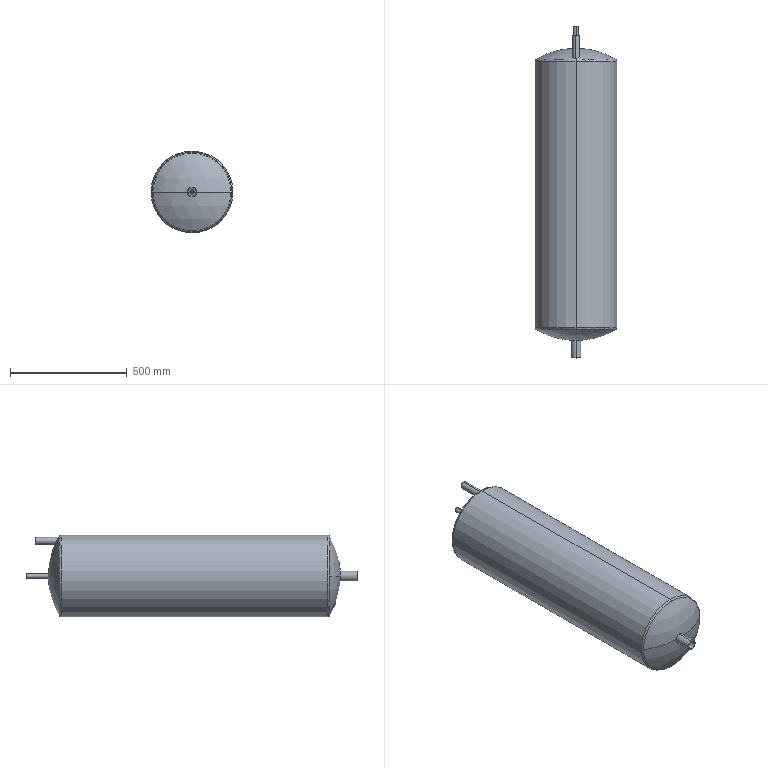Part | SolidWorks | features ICE 8, Revolution 1 | 1 solid | 35 faces | box 350 x 1420 x 350 mm | volume 7280812 mm3 | cylinder 16 | torus 8 | sphere 8 | plane 3 | commonest cylinder face diameters 10 x2 20 x2 26 x2 30 x2 37 x2 42 x2
STEP:
#1=CARTESIAN_POINT('',(0.,576.425,163.));
#2=VERTEX_POINT('',#1);
#3=CARTESIAN_POINT('',(0.,589.882,137.));
#4=VERTEX_POINT('',#3);
#5=CARTESIAN_POINT('',(0.,576.425,163.));
#6=CARTESIAN_POINT('',(-0.4541,576.425,163.));
#7=CARTESIAN_POINT('',(-0.9133,576.438,162.976));
#8=CARTESIAN_POINT('',(-1.814,576.488,162.881));
#9=CARTESIAN_POINT('',(-2.259,576.525,162.81));
#10=CARTESIAN_POINT('',(-3.136,576.624,162.624));
#11=CARTESIAN_POINT('',(-3.569,576.685,162.508));
#12=CARTESIAN_POINT('',(-4.425,576.831,162.232));
#13=CARTESIAN_POINT('',(-4.846,576.917,162.071));
#14=CARTESIAN_POINT('',(-6.062,577.201,161.534));
#15=CARTESIAN_POINT('',(-6.822,577.43,161.101));
#16=CARTESIAN_POINT('',(-7.888,577.829,160.343));
#17=CARTESIAN_POINT('',(-8.229,577.971,160.073));
#18=CARTESIAN_POINT('',(-8.873,578.268,159.51));
#19=CARTESIAN_POINT('',(-9.179,578.423,159.216));
#20=CARTESIAN_POINT('',(-9.757,578.746,158.601));
#21=CARTESIAN_POINT('',(-10.03,578.915,158.281));
#22=CARTESIAN_POINT('',(-10.544,579.264,157.616));
#23=CARTESIAN_POINT('',(-10.784,579.445,157.271));
#24=CARTESIAN_POINT('',(-11.446,579.996,156.219));
#25=CARTESIAN_POINT('',(-11.813,580.378,155.488));
#26=CARTESIAN_POINT('',(-12.258,580.972,154.349));
#27=CARTESIAN_POINT('',(-12.388,581.175,153.961));
#28=CARTESIAN_POINT('',(-12.612,581.582,153.179));
#29=CARTESIAN_POINT('',(-12.704,581.787,152.785));
#30=CARTESIAN_POINT('',(-12.926,582.403,151.6));
#31=CARTESIAN_POINT('',(-13.,582.817,150.802));
#32=CARTESIAN_POINT('',(-13.,583.442,149.594));
#33=CARTESIAN_POINT('',(-12.981,583.651,149.188));
#34=CARTESIAN_POINT('',(-12.905,584.067,148.382));
#35=CARTESIAN_POINT('',(-12.849,584.274,147.982));
#36=CARTESIAN_POINT('',(-12.698,584.684,147.187));
#37=CARTESIAN_POINT('',(-12.605,584.887,146.792));
#38=CARTESIAN_POINT('',(-12.378,585.29,146.007));
#39=CARTESIAN_POINT('',(-12.246,585.49,145.619));
#40=CARTESIAN_POINT('',(-11.799,586.074,144.481));
#41=CARTESIAN_POINT('',(-11.43,586.447,143.751));
#42=CARTESIAN_POINT('',(-10.766,586.984,142.702));
#43=CARTESIAN_POINT('',(-10.527,587.158,142.36));
#44=CARTESIAN_POINT('',(-10.008,587.499,141.692));
#45=CARTESIAN_POINT('',(-9.733,587.662,141.372));
#46=CARTESIAN_POINT('',(-8.863,588.131,140.452));
#47=CARTESIAN_POINT('',(-8.222,588.415,139.893));
#48=CARTESIAN_POINT('',(-7.162,588.797,139.142));
#49=CARTESIAN_POINT('',(-6.79,588.917,138.906));
#50=CARTESIAN_POINT('',(-6.023,589.137,138.471));
#51=CARTESIAN_POINT('',(-5.629,589.237,138.274));
#52=CARTESIAN_POINT('',(-4.42,589.506,137.743));
#53=CARTESIAN_POINT('',(-3.575,589.645,137.469));
#54=CARTESIAN_POINT('',(-2.246,589.787,137.188));
#55=CARTESIAN_POINT('',(-1.796,589.823,137.117));
#56=CARTESIAN_POINT('',(-0.8995,589.87,137.023));
#57=CARTESIAN_POINT('',(-0.4502,589.882,137.));
#58=CARTESIAN_POINT('',(0.,589.882,137.));
#59=B_SPLINE_CURVE_WITH_KNOTS('',3,(#5,#6,#7,#8,#9,#10,#11,#12,#13,#14,#15,#16,#17,#18,#19,#20,#21,#22,#23,#24,#25,#26,#27,#28,#29,#30,#31,#32,#33,#34,#35,#36,#37,#38,#39,#40,#41,#42,#43,#44,#45,#46,#47,#48,#49,#50,#51,#52,#53,#54,#55,#56,#57,#58),.UNSPECIFIED.,.F.,.F.,(4,2,2,2,2,2,2,2,2,2,2,2,2,2,2,2,2,2,2,2,2,2,2,2,2,2,4),(0.06034,0.06169,0.06303,0.06438,0.06573,0.06843,0.06978,0.07112,0.07247,0.07382,0.07652,0.07787,0.07921,0.08191,0.08326,0.08461,0.08596,0.08731,0.09,0.09135,0.0927,0.0954,0.09674,0.09809,0.1008,0.1021,0.1035),.UNSPECIFIED.);
#60=EDGE_CURVE('',#2,#4,#59,.T.);
#61=ORIENTED_EDGE('',*,*,#60,.T.);
#62=CARTESIAN_POINT('',(0.,680.,137.));
#63=VERTEX_POINT('',#62);
#64=CARTESIAN_POINT('',(0.,-700.001,137.));
#65=DIRECTION('',(0.,1.,0.));
#66=VECTOR('',#65,1000.);
#67=LINE('',#64,#66);
#68=EDGE_CURVE('',#4,#63,#67,.T.);
#69=ORIENTED_EDGE('',*,*,#68,.T.);
#70=CARTESIAN_POINT('',(0.,680.,163.));
#71=VERTEX_POINT('',#70);
#72=CARTESIAN_POINT('',(0.,680.,150.));
#73=DIRECTION('',(0.,1.,0.));
#74=DIRECTION('',(0.,0.,1.));
#75=AXIS2_PLACEMENT_3D('',#72,#73,#74);
#76=CIRCLE('',#75,13.);
#77=EDGE_CURVE('',#63,#71,#76,.T.);
#78=ORIENTED_EDGE('',*,*,#77,.T.);
#79=CARTESIAN_POINT('',(0.,-700.001,163.));
#80=DIRECTION('',(0.,1.,0.));
#81=VECTOR('',#80,1000.);
#82=LINE('',#79,#81);
#83=EDGE_CURVE('',#2,#71,#82,.T.);
#84=ORIENTED_EDGE('',*,*,#83,.F.);
#85=EDGE_LOOP('',(#61,#69,#78,#84));
#86=FACE_OUTER_BOUND('',#85,.T.);
#87=CARTESIAN_POINT('',(0.,-700.001,150.));
#88=DIRECTION('',(0.,1.,0.));
#89=DIRECTION('',(0.,0.,1.));
#90=AXIS2_PLACEMENT_3D('',#87,#88,#89);
#91=CYLINDRICAL_SURFACE('',#90,13.);
#92=ADVANCED_FACE('',(#86),#91,.F.);
#93=CARTESIAN_POINT('',(0.,581.042,165.));
#94=VERTEX_POINT('',#93);
#95=CARTESIAN_POINT('',(0.,596.28,135.));
#96=VERTEX_POINT('',#95);
#97=CARTESIAN_POINT('',(0.,581.042,165.));
#98=CARTESIAN_POINT('',(1.049,581.042,165.));
#99=CARTESIAN_POINT('',(2.08,581.099,164.891));
#100=CARTESIAN_POINT('',(3.602,581.266,164.57));
#101=CARTESIAN_POINT('',(4.108,581.336,164.436));
#102=CARTESIAN_POINT('',(5.093,581.502,164.118));
#103=CARTESIAN_POINT('',(5.572,581.597,163.936));
#104=CARTESIAN_POINT('',(6.504,581.81,163.526));
#105=CARTESIAN_POINT('',(6.957,581.928,163.299));
#106=CARTESIAN_POINT('',(7.837,582.187,162.8));
#107=CARTESIAN_POINT('',(8.267,582.329,162.526));
#108=CARTESIAN_POINT('',(9.493,582.78,161.657));
#109=CARTESIAN_POINT('',(10.235,583.116,161.009));
#110=CARTESIAN_POINT('',(11.242,583.667,159.943));
#111=CARTESIAN_POINT('',(11.561,583.86,159.57));
#112=CARTESIAN_POINT('',(12.154,584.255,158.804));
#113=CARTESIAN_POINT('',(12.429,584.458,158.41));
#114=CARTESIAN_POINT('',(13.193,585.08,157.201));
#115=CARTESIAN_POINT('',(13.62,585.515,156.356));
#116=CARTESIAN_POINT('',(14.312,586.42,154.59));
#117=CARTESIAN_POINT('',(14.568,586.879,153.692));
#118=CARTESIAN_POINT('',(14.826,587.577,152.324));
#119=CARTESIAN_POINT('',(14.891,587.811,151.864));
#120=CARTESIAN_POINT('',(14.978,588.283,150.938));
#121=CARTESIAN_POINT('',(15.,588.521,150.47));
#122=CARTESIAN_POINT('',(15.,589.232,149.069));
#123=CARTESIAN_POINT('',(14.914,589.7,148.146));
#124=CARTESIAN_POINT('',(14.657,590.391,146.778));
#125=CARTESIAN_POINT('',(14.55,590.62,146.325));
#126=CARTESIAN_POINT('',(14.292,591.074,145.423));
#127=CARTESIAN_POINT('',(14.141,591.301,144.974));
#128=CARTESIAN_POINT('',(13.622,591.968,143.648));
#129=CARTESIAN_POINT('',(13.195,592.392,142.804));
#130=CARTESIAN_POINT('',(12.433,592.997,141.595));
#131=CARTESIAN_POINT('',(12.159,593.194,141.202));
#132=CARTESIAN_POINT('',(11.566,593.576,140.437));
#133=CARTESIAN_POINT('',(11.247,593.763,140.063));
#134=CARTESIAN_POINT('',(10.232,594.3,138.987));
#135=CARTESIAN_POINT('',(9.489,594.622,138.34));
#136=CARTESIAN_POINT('',(8.272,595.051,137.477));
#137=CARTESIAN_POINT('',(7.849,595.185,137.208));
#138=CARTESIAN_POINT('',(6.968,595.434,136.707));
#139=CARTESIAN_POINT('',(6.506,595.549,136.475));
#140=CARTESIAN_POINT('',(5.098,595.856,135.856));
#141=CARTESIAN_POINT('',(4.123,596.013,135.541));
#142=CARTESIAN_POINT('',(2.604,596.172,135.219));
#143=CARTESIAN_POINT('',(2.086,596.213,135.136));
#144=CARTESIAN_POINT('',(1.041,596.267,135.027));
#145=CARTESIAN_POINT('',(0.5199,596.28,135.));
#146=CARTESIAN_POINT('',(0.,596.28,135.));
#147=B_SPLINE_CURVE_WITH_KNOTS('',3,(#97,#98,#99,#100,#101,#102,#103,#104,#105,#106,#107,#108,#109,#110,#111,#112,#113,#114,#115,#116,#117,#118,#119,#120,#121,#122,#123,#124,#125,#126,#127,#128,#129,#130,#131,#132,#133,#134,#135,#136,#137,#138,#139,#140,#141,#142,#143,#144,#145,#146),.UNSPECIFIED.,.F.,.F.,(4,2,2,2,2,2,2,2,2,2,2,2,2,2,2,2,2,2,2,2,2,2,2,2,4),(0.0299,0.033,0.03456,0.03611,0.03766,0.03921,0.04232,0.04387,0.04542,0.04853,0.05163,0.05318,0.05473,0.05784,0.05939,0.06094,0.06405,0.0656,0.06715,0.07026,0.07181,0.07336,0.07646,0.07802,0.07957),.UNSPECIFIED.);
#148=EDGE_CURVE('',#94,#96,#147,.T.);
#149=ORIENTED_EDGE('',*,*,#148,.T.);
#150=CARTESIAN_POINT('',(0.,680.,135.));
#151=VERTEX_POINT('',#150);
#152=CARTESIAN_POINT('',(0.,-700.001,135.));
#153=DIRECTION('',(0.,1.,0.));
#154=VECTOR('',#153,1000.);
#155=LINE('',#152,#154);
#156=EDGE_CURVE('',#96,#151,#155,.T.);
#157=ORIENTED_EDGE('',*,*,#156,.T.);
#158=CARTESIAN_POINT('',(0.,680.,165.));
#159=VERTEX_POINT('',#158);
#160=CARTESIAN_POINT('',(0.,680.,150.));
#161=DIRECTION('',(0.,1.,0.));
#162=DIRECTION('',(0.,0.,1.));
#163=AXIS2_PLACEMENT_3D('',#160,#161,#162);
#164=CIRCLE('',#163,15.);
#165=EDGE_CURVE('',#159,#151,#164,.T.);
#166=ORIENTED_EDGE('',*,*,#165,.F.);
#167=CARTESIAN_POINT('',(0.,-700.001,165.));
#168=DIRECTION('',(0.,1.,0.));
#169=VECTOR('',#168,1000.);
#170=LINE('',#167,#169);
#171=EDGE_CURVE('',#94,#159,#170,.T.);
#172=ORIENTED_EDGE('',*,*,#171,.F.);
#173=EDGE_LOOP('',(#149,#157,#166,#172));
#174=FACE_OUTER_BOUND('',#173,.T.);
#175=CARTESIAN_POINT('',(0.,-700.001,150.));
#176=DIRECTION('',(0.,1.,0.));
#177=DIRECTION('',(0.,0.,1.));
#178=AXIS2_PLACEMENT_3D('',#175,#176,#177);
#179=CYLINDRICAL_SURFACE('',#178,15.);
#180=ADVANCED_FACE('',(#174),#179,.T.);
#181=CARTESIAN_POINT('',(-5.,619.962,0.));
#182=VERTEX_POINT('',#181);
#183=CARTESIAN_POINT('',(0.,619.962,-5.));
#184=VERTEX_POINT('',#183);
#185=CARTESIAN_POINT('',(0.,619.962,0.));
#186=DIRECTION('',(0.,-1.,0.));
#187=DIRECTION('',(0.,0.,-1.));
#188=AXIS2_PLACEMENT_3D('',#185,#186,#187);
#189=CIRCLE('',#188,5.);
#190=EDGE_CURVE('',#182,#184,#189,.T.);
#191=ORIENTED_EDGE('',*,*,#190,.T.);
#192=CARTESIAN_POINT('',(0.,720.,-5.));
#193=VERTEX_POINT('',#192);
#194=CARTESIAN_POINT('',(0.,-700.001,-5.));
#195=DIRECTION('',(0.,1.,0.));
#196=VECTOR('',#195,1000.);
#197=LINE('',#194,#196);
#198=EDGE_CURVE('',#184,#193,#197,.T.);
#199=ORIENTED_EDGE('',*,*,#198,.T.);
#200=CARTESIAN_POINT('',(0.,720.,5.));
#201=VERTEX_POINT('',#200);
#202=CARTESIAN_POINT('',(0.,720.,0.));
#203=DIRECTION('',(0.,1.,0.));
#204=DIRECTION('',(0.,0.,1.));
#205=AXIS2_PLACEMENT_3D('',#202,#203,#204);
#206=CIRCLE('',#205,5.);
#207=EDGE_CURVE('',#193,#201,#206,.T.);
#208=ORIENTED_EDGE('',*,*,#207,.T.);
#209=CARTESIAN_POINT('',(0.,619.962,5.));
#210=VERTEX_POINT('',#209);
#211=CARTESIAN_POINT('',(0.,-700.001,5.));
#212=DIRECTION('',(0.,1.,0.));
#213=VECTOR('',#212,1000.);
#214=LINE('',#211,#213);
#215=EDGE_CURVE('',#210,#201,#214,.T.);
#216=ORIENTED_EDGE('',*,*,#215,.F.);
#217=CARTESIAN_POINT('',(0.,619.962,0.));
#218=DIRECTION('',(0.,-1.,0.));
#219=DIRECTION('',(0.,0.,-1.));
#220=AXIS2_PLACEMENT_3D('',#217,#218,#219);
#221=CIRCLE('',#220,5.);
#222=EDGE_CURVE('',#210,#182,#221,.T.);
#223=ORIENTED_EDGE('',*,*,#222,.T.);
#224=EDGE_LOOP('',(#191,#199,#208,#216,#223));
#225=FACE_OUTER_BOUND('',#224,.T.);
#226=CARTESIAN_POINT('',(0.,-700.001,0.));
#227=DIRECTION('',(0.,1.,0.));
#228=DIRECTION('',(0.,0.,1.));
#229=AXIS2_PLACEMENT_3D('',#226,#227,#228);
#230=CYLINDRICAL_SURFACE('',#229,5.);
#231=ADVANCED_FACE('',(#225),#230,.F.);
#232=CARTESIAN_POINT('',(10.,624.849,0.));
#233=VERTEX_POINT('',#232);
#234=CARTESIAN_POINT('',(0.,624.849,-10.));
#235=VERTEX_POINT('',#234);
#236=CARTESIAN_POINT('',(0.,624.849,0.));
#237=DIRECTION('',(0.,1.,0.));
#238=DIRECTION('',(0.,0.,-1.));
#239=AXIS2_PLACEMENT_3D('',#236,#237,#238);
#240=CIRCLE('',#239,10.);
#241=EDGE_CURVE('',#233,#235,#240,.T.);
#242=ORIENTED_EDGE('',*,*,#241,.T.);
#243=CARTESIAN_POINT('',(0.,720.,-10.));
#244=VERTEX_POINT('',#243);
#245=CARTESIAN_POINT('',(0.,-700.001,-10.));
#246=DIRECTION('',(0.,1.,0.));
#247=VECTOR('',#246,1000.);
#248=LINE('',#245,#247);
#249=EDGE_CURVE('',#235,#244,#248,.T.);
#250=ORIENTED_EDGE('',*,*,#249,.T.);
#251=CARTESIAN_POINT('',(0.,720.,10.));
#252=VERTEX_POINT('',#251);
#253=CARTESIAN_POINT('',(0.,720.,0.));
#254=DIRECTION('',(0.,1.,0.));
#255=DIRECTION('',(0.,0.,1.));
#256=AXIS2_PLACEMENT_3D('',#253,#254,#255);
#257=CIRCLE('',#256,10.);
#258=EDGE_CURVE('',#252,#244,#257,.T.);
#259=ORIENTED_EDGE('',*,*,#258,.F.);
#260=CARTESIAN_POINT('',(0.,624.849,10.));
#261=VERTEX_POINT('',#260);
#262=CARTESIAN_POINT('',(0.,-700.001,10.));
#263=DIRECTION('',(0.,1.,0.));
#264=VECTOR('',#263,1000.);
#265=LINE('',#262,#264);
#266=EDGE_CURVE('',#261,#252,#265,.T.);
#267=ORIENTED_EDGE('',*,*,#266,.F.);
#268=CARTESIAN_POINT('',(0.,624.849,0.));
#269=DIRECTION('',(0.,1.,0.));
#270=DIRECTION('',(0.,0.,-1.));
#271=AXIS2_PLACEMENT_3D('',#268,#269,#270);
#272=CIRCLE('',#271,10.);
#273=EDGE_CURVE('',#261,#233,#272,.T.);
#274=ORIENTED_EDGE('',*,*,#273,.T.);
#275=EDGE_LOOP('',(#242,#250,#259,#267,#274));
#276=FACE_OUTER_BOUND('',#275,.T.);
#277=CARTESIAN_POINT('',(0.,-700.001,0.));
#278=DIRECTION('',(0.,1.,0.));
#279=DIRECTION('',(0.,0.,1.));
#280=AXIS2_PLACEMENT_3D('',#277,#278,#279);
#281=CYLINDRICAL_SURFACE('',#280,10.);
#282=ADVANCED_FACE('',(#276),#281,.T.);
#283=CARTESIAN_POINT('',(0.,-619.476,18.5));
#284=VERTEX_POINT('',#283);
#285=CARTESIAN_POINT('',(-18.5,-619.476,0.));
#286=VERTEX_POINT('',#285);
#287=CARTESIAN_POINT('',(0.,-619.476,0.));
#288=DIRECTION('',(0.,-1.,0.));
#289=DIRECTION('',(0.,0.,1.));
#290=AXIS2_PLACEMENT_3D('',#287,#288,#289);
#291=CIRCLE('',#290,18.5);
#292=EDGE_CURVE('',#284,#286,#291,.T.);
#293=ORIENTED_EDGE('',*,*,#292,.F.);
#294=CARTESIAN_POINT('',(0.,-700.,18.5));
#295=VERTEX_POINT('',#294);
#296=CARTESIAN_POINT('',(0.,625.001,18.5));
#297=DIRECTION('',(0.,-1.,0.));
#298=VECTOR('',#297,1000.);
#299=LINE('',#296,#298);
#300=EDGE_CURVE('',#284,#295,#299,.T.);
#301=ORIENTED_EDGE('',*,*,#300,.T.);
#302=CARTESIAN_POINT('',(0.,-700.,-18.5));
#303=VERTEX_POINT('',#302);
#304=CARTESIAN_POINT('',(0.,-700.,0.));
#305=DIRECTION('',(0.,1.,0.));
#306=DIRECTION('',(0.,0.,1.));
#307=AXIS2_PLACEMENT_3D('',#304,#305,#306);
#308=CIRCLE('',#307,18.5);
#309=EDGE_CURVE('',#303,#295,#308,.T.);
#310=ORIENTED_EDGE('',*,*,#309,.F.);
#311=CARTESIAN_POINT('',(0.,-619.476,-18.5));
#312=VERTEX_POINT('',#311);
#313=CARTESIAN_POINT('',(0.,625.001,-18.5));
#314=DIRECTION('',(0.,-1.,0.));
#315=VECTOR('',#314,1000.);
#316=LINE('',#313,#315);
#317=EDGE_CURVE('',#312,#303,#316,.T.);
#318=ORIENTED_EDGE('',*,*,#317,.F.);
#319=CARTESIAN_POINT('',(0.,-619.476,0.));
#320=DIRECTION('',(0.,-1.,0.));
#321=DIRECTION('',(0.,0.,1.));
#322=AXIS2_PLACEMENT_3D('',#319,#320,#321);
#323=CIRCLE('',#322,18.5);
#324=EDGE_CURVE('',#286,#312,#323,.T.);
#325=ORIENTED_EDGE('',*,*,#324,.F.);
#326=EDGE_LOOP('',(#293,#301,#310,#318,#325));
#327=FACE_OUTER_BOUND('',#326,.T.);
#328=CARTESIAN_POINT('',(0.,625.001,0.));
#329=DIRECTION('',(0.,-1.,0.));
#330=DIRECTION('',(0.,0.,-1.));
#331=AXIS2_PLACEMENT_3D('',#328,#329,#330);
#332=CYLINDRICAL_SURFACE('',#331,18.5);
#333=ADVANCED_FACE('',(#327),#332,.F.);
#334=CARTESIAN_POINT('',(21.,-624.334,0.));
#335=VERTEX_POINT('',#334);
#336=CARTESIAN_POINT('',(0.,-624.334,21.));
#337=VERTEX_POINT('',#336);
#338=CARTESIAN_POINT('',(0.,-624.334,0.));
#339=DIRECTION('',(0.,-1.,0.));
#340=DIRECTION('',(0.,0.,1.));
#341=AXIS2_PLACEMENT_3D('',#338,#339,#340);
#342=CIRCLE('',#341,21.);
#343=EDGE_CURVE('',#335,#337,#342,.T.);
#344=ORIENTED_EDGE('',*,*,#343,.T.);
#345=CARTESIAN_POINT('',(0.,-700.,21.));
#346=VERTEX_POINT('',#345);
#347=CARTESIAN_POINT('',(0.,625.001,21.));
#348=DIRECTION('',(0.,-1.,0.));
#349=VECTOR('',#348,1000.);
#350=LINE('',#347,#349);
#351=EDGE_CURVE('',#337,#346,#350,.T.);
#352=ORIENTED_EDGE('',*,*,#351,.T.);
#353=CARTESIAN_POINT('',(0.,-700.,-21.));
#354=VERTEX_POINT('',#353);
#355=CARTESIAN_POINT('',(0.,-700.,0.));
#356=DIRECTION('',(0.,1.,0.));
#357=DIRECTION('',(0.,0.,1.));
#358=AXIS2_PLACEMENT_3D('',#355,#356,#357);
#359=CIRCLE('',#358,21.);
#360=EDGE_CURVE('',#346,#354,#359,.T.);
#361=ORIENTED_EDGE('',*,*,#360,.T.);
#362=CARTESIAN_POINT('',(0.,-624.334,-21.));
#363=VERTEX_POINT('',#362);
#364=CARTESIAN_POINT('',(0.,625.001,-21.));
#365=DIRECTION('',(0.,-1.,0.));
#366=VECTOR('',#365,1000.);
#367=LINE('',#364,#366);
#368=EDGE_CURVE('',#363,#354,#367,.T.);
#369=ORIENTED_EDGE('',*,*,#368,.F.);
#370=CARTESIAN_POINT('',(0.,-624.334,0.));
#371=DIRECTION('',(0.,-1.,0.));
#372=DIRECTION('',(0.,0.,1.));
#373=AXIS2_PLACEMENT_3D('',#370,#371,#372);
#374=CIRCLE('',#373,21.);
#375=EDGE_CURVE('',#363,#335,#374,.T.);
#376=ORIENTED_EDGE('',*,*,#375,.T.);
#377=EDGE_LOOP('',(#344,#352,#361,#369,#376));
#378=FACE_OUTER_BOUND('',#377,.T.);
#379=CARTESIAN_POINT('',(0.,625.001,0.));
#380=DIRECTION('',(0.,-1.,0.));
#381=DIRECTION('',(0.,0.,-1.));
#382=AXIS2_PLACEMENT_3D('',#379,#380,#381);
#383=CYLINDRICAL_SURFACE('',#382,21.);
#384=ADVANCED_FACE('',(#378),#383,.T.);
#385=CARTESIAN_POINT('',(170.13,578.039,0.));
#386=VERTEX_POINT('',#385);
#387=CARTESIAN_POINT('',(0.,578.039,170.13));
#388=VERTEX_POINT('',#387);
#389=CARTESIAN_POINT('',(0.,578.039,0.));
#390=DIRECTION('',(0.,-1.,0.));
#391=DIRECTION('',(0.,0.,-1.));
#392=AXIS2_PLACEMENT_3D('',#389,#390,#391);
#393=CIRCLE('',#392,170.13);
#394=EDGE_CURVE('',#386,#388,#393,.T.);
#395=ORIENTED_EDGE('',*,*,#394,.T.);
#396=CARTESIAN_POINT('',(0.,569.455,175.));
#397=VERTEX_POINT('',#396);
#398=CARTESIAN_POINT('',(0.,569.455,165.));
#399=DIRECTION('',(1.,0.,0.));
#400=DIRECTION('',(0.,0.,-1.));
#401=AXIS2_PLACEMENT_3D('',#398,#399,#400);
#402=CIRCLE('',#401,10.);
#403=EDGE_CURVE('',#388,#397,#402,.T.);
#404=ORIENTED_EDGE('',*,*,#403,.T.);
#405=CARTESIAN_POINT('',(0.,569.455,-175.));
#406=VERTEX_POINT('',#405);
#407=CARTESIAN_POINT('',(0.,569.455,0.));
#408=DIRECTION('',(0.,-1.,0.));
#409=DIRECTION('',(0.,0.,-1.));
#410=AXIS2_PLACEMENT_3D('',#407,#408,#409);
#411=CIRCLE('',#410,175.);
#412=EDGE_CURVE('',#406,#397,#411,.T.);
#413=ORIENTED_EDGE('',*,*,#412,.F.);
#414=CARTESIAN_POINT('',(0.,578.039,-170.13));
#415=VERTEX_POINT('',#414);
#416=CARTESIAN_POINT('',(0.,569.455,-165.));
#417=DIRECTION('',(-1.,0.,0.));
#418=DIRECTION('',(0.,0.,1.));
#419=AXIS2_PLACEMENT_3D('',#416,#417,#418);
#420=CIRCLE('',#419,10.);
#421=EDGE_CURVE('',#415,#406,#420,.T.);
#422=ORIENTED_EDGE('',*,*,#421,.F.);
#423=CARTESIAN_POINT('',(0.,578.039,0.));
#424=DIRECTION('',(0.,-1.,0.));
#425=DIRECTION('',(0.,0.,-1.));
#426=AXIS2_PLACEMENT_3D('',#423,#424,#425);
#427=CIRCLE('',#426,170.13);
#428=EDGE_CURVE('',#415,#386,#427,.T.);
#429=ORIENTED_EDGE('',*,*,#428,.T.);
#430=EDGE_LOOP('',(#395,#404,#413,#422,#429));
#431=FACE_OUTER_BOUND('',#430,.T.);
#432=CARTESIAN_POINT('',(0.,569.455,0.));
#433=DIRECTION('',(0.,-1.,0.));
#434=DIRECTION('',(0.,0.,-1.));
#435=AXIS2_PLACEMENT_3D('',#432,#433,#434);
#436=TOROIDAL_SURFACE('',#435,165.,10.);
#437=ADVANCED_FACE('',(#431),#436,.T.);
#438=ORIENTED_EDGE('',*,*,#412,.T.);
#439=CARTESIAN_POINT('',(0.,-569.455,175.));
#440=VERTEX_POINT('',#439);
#441=CARTESIAN_POINT('',(0.,0.,175.));
#442=DIRECTION('',(0.,-1.,0.));
#443=VECTOR('',#442,1000.);
#444=LINE('',#441,#443);
#445=EDGE_CURVE('',#397,#440,#444,.T.);
#446=ORIENTED_EDGE('',*,*,#445,.T.);
#447=CARTESIAN_POINT('',(0.,-569.455,-175.));
#448=VERTEX_POINT('',#447);
#449=CARTESIAN_POINT('',(0.,-569.455,0.));
#450=DIRECTION('',(0.,-1.,0.));
#451=DIRECTION('',(0.,0.,-1.));
#452=AXIS2_PLACEMENT_3D('',#449,#450,#451);
#453=CIRCLE('',#452,175.);
#454=EDGE_CURVE('',#448,#440,#453,.T.);
#455=ORIENTED_EDGE('',*,*,#454,.F.);
#456=CARTESIAN_POINT('',(0.,0.,-175.));
#457=DIRECTION('',(0.,-1.,0.));
#458=VECTOR('',#457,1000.);
#459=LINE('',#456,#458);
#460=EDGE_CURVE('',#406,#448,#459,.T.);
#461=ORIENTED_EDGE('',*,*,#460,.F.);
#462=EDGE_LOOP('',(#438,#446,#455,#461));
#463=FACE_OUTER_BOUND('',#462,.T.);
#464=CARTESIAN_POINT('',(0.,0.,0.));
#465=DIRECTION('',(0.,-1.,0.));
#466=DIRECTION('',(0.,0.,-1.));
#467=AXIS2_PLACEMENT_3D('',#464,#465,#466);
#468=CYLINDRICAL_SURFACE('',#467,175.);
#469=ADVANCED_FACE('',(#463),#468,.T.);
#470=ORIENTED_EDGE('',*,*,#454,.T.);
#471=CARTESIAN_POINT('',(0.,-578.039,170.13));
#472=VERTEX_POINT('',#471);
#473=CARTESIAN_POINT('',(0.,-569.455,165.));
#474=DIRECTION('',(1.,0.,0.));
#475=DIRECTION('',(0.,0.,-1.));
#476=AXIS2_PLACEMENT_3D('',#473,#474,#475);
#477=CIRCLE('',#476,10.);
#478=EDGE_CURVE('',#440,#472,#477,.T.);
#479=ORIENTED_EDGE('',*,*,#478,.T.);
#480=CARTESIAN_POINT('',(170.13,-578.039,0.));
#481=VERTEX_POINT('',#480);
#482=CARTESIAN_POINT('',(0.,-578.039,0.));
#483=DIRECTION('',(0.,-1.,0.));
#484=DIRECTION('',(0.,0.,-1.));
#485=AXIS2_PLACEMENT_3D('',#482,#483,#484);
#486=CIRCLE('',#485,170.13);
#487=EDGE_CURVE('',#481,#472,#486,.T.);
#488=ORIENTED_EDGE('',*,*,#487,.F.);
#489=CARTESIAN_POINT('',(0.,-578.039,-170.13));
#490=VERTEX_POINT('',#489);
#491=CARTESIAN_POINT('',(0.,-578.039,0.));
#492=DIRECTION('',(0.,-1.,0.));
#493=DIRECTION('',(0.,0.,-1.));
#494=AXIS2_PLACEMENT_3D('',#491,#492,#493);
#495=CIRCLE('',#494,170.13);
#496=EDGE_CURVE('',#490,#481,#495,.T.);
#497=ORIENTED_EDGE('',*,*,#496,.F.);
#498=CARTESIAN_POINT('',(0.,-569.455,-165.));
#499=DIRECTION('',(-1.,0.,0.));
#500=DIRECTION('',(0.,0.,1.));
#501=AXIS2_PLACEMENT_3D('',#498,#499,#500);
#502=CIRCLE('',#501,10.);
#503=EDGE_CURVE('',#448,#490,#502,.T.);
#504=ORIENTED_EDGE('',*,*,#503,.F.);
#505=EDGE_LOOP('',(#470,#479,#488,#497,#504));
#506=FACE_OUTER_BOUND('',#505,.T.);
#507=CARTESIAN_POINT('',(0.,-569.455,0.));
#508=DIRECTION('',(0.,-1.,0.));
#509=DIRECTION('',(0.,0.,-1.));
#510=AXIS2_PLACEMENT_3D('',#507,#508,#509);
#511=TOROIDAL_SURFACE('',#510,165.,10.);
#512=ADVANCED_FACE('',(#506),#511,.T.);
#513=ORIENTED_EDGE('',*,*,#148,.F.);
#514=CARTESIAN_POINT('',(0.,596.28,135.));
#515=CARTESIAN_POINT('',(-0.52,596.28,135.));
#516=CARTESIAN_POINT('',(-1.039,596.267,135.027));
#517=CARTESIAN_POINT('',(-2.074,596.214,135.135));
#518=CARTESIAN_POINT('',(-2.593,596.173,135.216));
#519=CARTESIAN_POINT('',(-4.128,596.012,135.541));
#520=CARTESIAN_POINT('',(-5.108,595.855,135.859));
#521=CARTESIAN_POINT('',(-6.513,595.548,136.478));
#522=CARTESIAN_POINT('',(-6.973,595.433,136.71));
#523=CARTESIAN_POINT('',(-7.86,595.182,137.214));
#524=CARTESIAN_POINT('',(-8.285,595.047,137.486));
#525=CARTESIAN_POINT('',(-9.101,594.759,138.066));
#526=CARTESIAN_POINT('',(-9.491,594.605,138.374));
#527=CARTESIAN_POINT('',(-10.239,594.28,139.027));
#528=CARTESIAN_POINT('',(-10.598,594.107,139.373));
#529=CARTESIAN_POINT('',(-11.611,593.569,140.452));
#530=CARTESIAN_POINT('',(-12.2,593.185,141.22));
#531=CARTESIAN_POINT('',(-13.219,592.37,142.847));
#532=CARTESIAN_POINT('',(-13.651,591.937,143.71));
#533=CARTESIAN_POINT('',(-14.164,591.268,145.04));
#534=CARTESIAN_POINT('',(-14.314,591.04,145.492));
#535=CARTESIAN_POINT('',(-14.569,590.583,146.398));
#536=CARTESIAN_POINT('',(-14.673,590.354,146.853));
#537=CARTESIAN_POINT('',(-14.923,589.661,148.223));
#538=CARTESIAN_POINT('',(-15.004,589.195,149.143));
#539=CARTESIAN_POINT('',(-14.998,588.488,150.535));
#540=CARTESIAN_POINT('',(-14.974,588.25,151.002));
#541=CARTESIAN_POINT('',(-14.882,587.777,151.932));
#542=CARTESIAN_POINT('',(-14.815,587.543,152.391));
#543=CARTESIAN_POINT('',(-14.551,586.846,153.757));
#544=CARTESIAN_POINT('',(-14.292,586.39,154.649));
#545=CARTESIAN_POINT('',(-13.774,585.719,155.958));
#546=CARTESIAN_POINT('',(-13.579,585.497,156.391));
#547=CARTESIAN_POINT('',(-13.146,585.06,157.24));
#548=CARTESIAN_POINT('',(-12.91,584.848,157.652));
#549=CARTESIAN_POINT('',(-12.145,584.229,158.855));
#550=CARTESIAN_POINT('',(-11.558,583.839,159.61));
#551=CARTESIAN_POINT('',(-10.555,583.292,160.669));
#552=CARTESIAN_POINT('',(-10.198,583.115,161.011));
#553=CARTESIAN_POINT('',(-9.447,582.778,161.662));
#554=CARTESIAN_POINT('',(-9.057,582.619,161.967));
#555=CARTESIAN_POINT('',(-7.841,582.174,162.826));
#556=CARTESIAN_POINT('',(-6.971,581.917,163.321));
#557=CARTESIAN_POINT('',(-5.569,581.596,163.937));
#558=CARTESIAN_POINT('',(-5.082,581.5,164.122));
#559=CARTESIAN_POINT('',(-4.1,581.335,164.438));
#560=CARTESIAN_POINT('',(-3.603,581.266,164.57));
#561=CARTESIAN_POINT('',(-2.595,581.156,164.783));
#562=CARTESIAN_POINT('',(-2.085,581.114,164.863));
#563=CARTESIAN_POINT('',(-1.31,581.071,164.945));
#564=CARTESIAN_POINT('',(-1.05,581.06,164.966));
#565=CARTESIAN_POINT('',(-0.5263,581.046,164.993));
#566=CARTESIAN_POINT('',(-0.2622,581.042,165.));
#567=CARTESIAN_POINT('',(0.,581.042,165.));
#568=B_SPLINE_CURVE_WITH_KNOTS('',3,(#514,#515,#516,#517,#518,#519,#520,#521,#522,#523,#524,#525,#526,#527,#528,#529,#530,#531,#532,#533,#534,#535,#536,#537,#538,#539,#540,#541,#542,#543,#544,#545,#546,#547,#548,#549,#550,#551,#552,#553,#554,#555,#556,#557,#558,#559,#560,#561,#562,#563,#564,#565,#566,#567),.UNSPECIFIED.,.F.,.F.,(4,2,2,2,2,2,2,2,2,2,2,2,2,2,2,2,2,2,2,2,2,2,2,2,2,2,4),(0.07957,0.08112,0.08267,0.08578,0.08733,0.08888,0.09043,0.09199,0.09509,0.0982,0.09975,0.1013,0.1044,0.106,0.1075,0.1106,0.1122,0.1137,0.1168,0.1184,0.1199,0.123,0.1246,0.1261,0.1277,0.1285,0.1292),.UNSPECIFIED.);
#569=EDGE_CURVE('',#96,#94,#568,.T.);
#570=ORIENTED_EDGE('',*,*,#569,.F.);
#571=EDGE_LOOP('',(#513,#570));
#572=FACE_BOUND('',#571,.T.);
#573=CARTESIAN_POINT('',(-10.,624.849,0.));
#574=VERTEX_POINT('',#573);
#575=CARTESIAN_POINT('',(0.,624.849,0.));
#576=DIRECTION('',(0.,1.,0.));
#577=DIRECTION('',(0.,0.,-1.));
#578=AXIS2_PLACEMENT_3D('',#575,#576,#577);
#579=CIRCLE('',#578,10.);
#580=EDGE_CURVE('',#574,#261,#579,.T.);
#581=ORIENTED_EDGE('',*,*,#580,.F.);
#582=CARTESIAN_POINT('',(-170.13,578.039,0.));
#583=VERTEX_POINT('',#582);
#584=CARTESIAN_POINT('',(0.,293.348,0.));
#585=DIRECTION('',(0.,0.,1.));
#586=DIRECTION('',(1.,0.,0.));
#587=AXIS2_PLACEMENT_3D('',#584,#585,#586);
#588=CIRCLE('',#587,331.652);
#589=EDGE_CURVE('',#574,#583,#588,.T.);
#590=ORIENTED_EDGE('',*,*,#589,.T.);
#591=CARTESIAN_POINT('',(0.,578.039,0.));
#592=DIRECTION('',(0.,-1.,0.));
#593=DIRECTION('',(0.,0.,-1.));
#594=AXIS2_PLACEMENT_3D('',#591,#592,#593);
#595=CIRCLE('',#594,170.13);
#596=EDGE_CURVE('',#388,#583,#595,.T.);
#597=ORIENTED_EDGE('',*,*,#596,.F.);
#598=ORIENTED_EDGE('',*,*,#394,.F.);
#599=CARTESIAN_POINT('',(0.,293.348,0.));
#600=DIRECTION('',(0.,0.,-1.));
#601=DIRECTION('',(-1.,0.,0.));
#602=AXIS2_PLACEMENT_3D('',#599,#600,#601);
#603=CIRCLE('',#602,331.652);
#604=EDGE_CURVE('',#233,#386,#603,.T.);
#605=ORIENTED_EDGE('',*,*,#604,.F.);
#606=ORIENTED_EDGE('',*,*,#273,.F.);
#607=EDGE_LOOP('',(#581,#590,#597,#598,#605,#606));
#608=FACE_OUTER_BOUND('',#607,.T.);
#609=CARTESIAN_POINT('',(0.,293.348,0.));
#610=DIRECTION('',(0.,0.,1.));
#611=DIRECTION('',(1.,0.,0.));
#612=AXIS2_PLACEMENT_3D('',#609,#610,#611);
#613=SPHERICAL_SURFACE('',#612,331.652);
#614=ADVANCED_FACE('',(#572,#608),#613,.T.);
#615=CARTESIAN_POINT('',(-170.13,-578.039,0.));
#616=VERTEX_POINT('',#615);
#617=CARTESIAN_POINT('',(0.,-578.039,0.));
#618=DIRECTION('',(0.,-1.,0.));
#619=DIRECTION('',(0.,0.,-1.));
#620=AXIS2_PLACEMENT_3D('',#617,#618,#619);
#621=CIRCLE('',#620,170.13);
#622=EDGE_CURVE('',#616,#490,#621,.T.);
#623=ORIENTED_EDGE('',*,*,#622,.T.);
#624=ORIENTED_EDGE('',*,*,#496,.T.);
#625=CARTESIAN_POINT('',(0.,-293.348,0.));
#626=DIRECTION('',(0.,0.,-1.));
#627=DIRECTION('',(-1.,0.,0.));
#628=AXIS2_PLACEMENT_3D('',#625,#626,#627);
#629=CIRCLE('',#628,331.652);
#630=EDGE_CURVE('',#481,#335,#629,.T.);
#631=ORIENTED_EDGE('',*,*,#630,.T.);
#632=ORIENTED_EDGE('',*,*,#375,.F.);
#633=CARTESIAN_POINT('',(-21.,-624.334,0.));
#634=VERTEX_POINT('',#633);
#635=CARTESIAN_POINT('',(0.,-624.334,0.));
#636=DIRECTION('',(0.,-1.,0.));
#637=DIRECTION('',(0.,0.,1.));
#638=AXIS2_PLACEMENT_3D('',#635,#636,#637);
#639=CIRCLE('',#638,21.);
#640=EDGE_CURVE('',#634,#363,#639,.T.);
#641=ORIENTED_EDGE('',*,*,#640,.F.);
#642=CARTESIAN_POINT('',(0.,-293.348,0.));
#643=DIRECTION('',(0.,0.,1.));
#644=DIRECTION('',(1.,0.,0.));
#645=AXIS2_PLACEMENT_3D('',#642,#643,#644);
#646=CIRCLE('',#645,331.652);
#647=EDGE_CURVE('',#616,#634,#646,.T.);
#648=ORIENTED_EDGE('',*,*,#647,.F.);
#649=EDGE_LOOP('',(#623,#624,#631,#632,#641,#648));
#650=FACE_OUTER_BOUND('',#649,.T.);
#651=CARTESIAN_POINT('',(0.,-293.348,0.));
#652=DIRECTION('',(0.,0.,-1.));
#653=DIRECTION('',(-1.,0.,0.));
#654=AXIS2_PLACEMENT_3D('',#651,#652,#653);
#655=SPHERICAL_SURFACE('',#654,331.652);
#656=ADVANCED_FACE('',(#650),#655,.T.);
#657=CARTESIAN_POINT('',(0.,-566.603,170.));
#658=VERTEX_POINT('',#657);
#659=CARTESIAN_POINT('',(0.,-566.603,-170.));
#660=VERTEX_POINT('',#659);
#661=CARTESIAN_POINT('',(0.,-566.603,0.));
#662=DIRECTION('',(0.,-1.,0.));
#663=DIRECTION('',(0.,0.,-1.));
#664=AXIS2_PLACEMENT_3D('',#661,#662,#663);
#665=CIRCLE('',#664,170.);
#666=EDGE_CURVE('',#658,#660,#665,.T.);
#667=ORIENTED_EDGE('',*,*,#666,.F.);
#668=CARTESIAN_POINT('',(0.,-575.233,165.053));
#669=VERTEX_POINT('',#668);
#670=CARTESIAN_POINT('',(0.,-566.603,160.));
#671=DIRECTION('',(1.,0.,0.));
#672=DIRECTION('',(0.,0.,-1.));
#673=AXIS2_PLACEMENT_3D('',#670,#671,#672);
#674=CIRCLE('',#673,10.);
#675=EDGE_CURVE('',#658,#669,#674,.T.);
#676=ORIENTED_EDGE('',*,*,#675,.T.);
#677=CARTESIAN_POINT('',(-165.053,-575.233,0.));
#678=VERTEX_POINT('',#677);
#679=CARTESIAN_POINT('',(0.,-575.233,0.));
#680=DIRECTION('',(0.,-1.,0.));
#681=DIRECTION('',(0.,0.,-1.));
#682=AXIS2_PLACEMENT_3D('',#679,#680,#681);
#683=CIRCLE('',#682,165.053);
#684=EDGE_CURVE('',#669,#678,#683,.T.);
#685=ORIENTED_EDGE('',*,*,#684,.T.);
#686=CARTESIAN_POINT('',(0.,-575.233,-165.053));
#687=VERTEX_POINT('',#686);
#688=CARTESIAN_POINT('',(0.,-575.233,0.));
#689=DIRECTION('',(0.,-1.,0.));
#690=DIRECTION('',(0.,0.,-1.));
#691=AXIS2_PLACEMENT_3D('',#688,#689,#690);
#692=CIRCLE('',#691,165.053);
#693=EDGE_CURVE('',#678,#687,#692,.T.);
#694=ORIENTED_EDGE('',*,*,#693,.T.);
#695=CARTESIAN_POINT('',(0.,-566.603,-160.));
#696=DIRECTION('',(-1.,0.,0.));
#697=DIRECTION('',(0.,0.,1.));
#698=AXIS2_PLACEMENT_3D('',#695,#696,#697);
#699=CIRCLE('',#698,10.);
#700=EDGE_CURVE('',#660,#687,#699,.T.);
#701=ORIENTED_EDGE('',*,*,#700,.F.);
#702=EDGE_LOOP('',(#667,#676,#685,#694,#701));
#703=FACE_OUTER_BOUND('',#702,.T.);
#704=CARTESIAN_POINT('',(0.,-566.603,0.));
#705=DIRECTION('',(0.,-1.,0.));
#706=DIRECTION('',(0.,0.,-1.));
#707=AXIS2_PLACEMENT_3D('',#704,#705,#706);
#708=TOROIDAL_SURFACE('',#707,160.,10.);
#709=ADVANCED_FACE('',(#703),#708,.F.);
#710=CARTESIAN_POINT('',(0.,566.603,170.));
#711=VERTEX_POINT('',#710);
#712=CARTESIAN_POINT('',(0.,566.603,-170.));
#713=VERTEX_POINT('',#712);
#714=CARTESIAN_POINT('',(0.,566.603,0.));
#715=DIRECTION('',(0.,-1.,0.));
#716=DIRECTION('',(0.,0.,-1.));
#717=AXIS2_PLACEMENT_3D('',#714,#715,#716);
#718=CIRCLE('',#717,170.);
#719=EDGE_CURVE('',#711,#713,#718,.T.);
#720=ORIENTED_EDGE('',*,*,#719,.F.);
#721=CARTESIAN_POINT('',(0.,0.,170.));
#722=DIRECTION('',(0.,-1.,0.));
#723=VECTOR('',#722,1000.);
#724=LINE('',#721,#723);
#725=EDGE_CURVE('',#711,#658,#724,.T.);
#726=ORIENTED_EDGE('',*,*,#725,.T.);
#727=ORIENTED_EDGE('',*,*,#666,.T.);
#728=CARTESIAN_POINT('',(0.,0.,-170.));
#729=DIRECTION('',(0.,-1.,0.));
#730=VECTOR('',#729,1000.);
#731=LINE('',#728,#730);
#732=EDGE_CURVE('',#713,#660,#731,.T.);
#733=ORIENTED_EDGE('',*,*,#732,.F.);
#734=EDGE_LOOP('',(#720,#726,#727,#733));
#735=FACE_OUTER_BOUND('',#734,.T.);
#736=CARTESIAN_POINT('',(0.,0.,0.));
#737=DIRECTION('',(0.,-1.,0.));
#738=DIRECTION('',(0.,0.,-1.));
#739=AXIS2_PLACEMENT_3D('',#736,#737,#738);
#740=CYLINDRICAL_SURFACE('',#739,170.);
#741=ADVANCED_FACE('',(#735),#740,.F.);
#742=CARTESIAN_POINT('',(0.,575.233,165.053));
#743=VERTEX_POINT('',#742);
#744=CARTESIAN_POINT('',(-165.053,575.233,0.));
#745=VERTEX_POINT('',#744);
#746=CARTESIAN_POINT('',(0.,575.233,0.));
#747=DIRECTION('',(0.,-1.,0.));
#748=DIRECTION('',(0.,0.,-1.));
#749=AXIS2_PLACEMENT_3D('',#746,#747,#748);
#750=CIRCLE('',#749,165.053);
#751=EDGE_CURVE('',#743,#745,#750,.T.);
#752=ORIENTED_EDGE('',*,*,#751,.F.);
#753=CARTESIAN_POINT('',(0.,566.603,160.));
#754=DIRECTION('',(1.,0.,0.));
#755=DIRECTION('',(0.,0.,-1.));
#756=AXIS2_PLACEMENT_3D('',#753,#754,#755);
#757=CIRCLE('',#756,10.);
#758=EDGE_CURVE('',#743,#711,#757,.T.);
#759=ORIENTED_EDGE('',*,*,#758,.T.);
#760=ORIENTED_EDGE('',*,*,#719,.T.);
#761=CARTESIAN_POINT('',(0.,575.233,-165.053));
#762=VERTEX_POINT('',#761);
#763=CARTESIAN_POINT('',(0.,566.603,-160.));
#764=DIRECTION('',(-1.,0.,0.));
#765=DIRECTION('',(0.,0.,1.));
#766=AXIS2_PLACEMENT_3D('',#763,#764,#765);
#767=CIRCLE('',#766,10.);
#768=EDGE_CURVE('',#762,#713,#767,.T.);
#769=ORIENTED_EDGE('',*,*,#768,.F.);
#770=CARTESIAN_POINT('',(0.,575.233,0.));
#771=DIRECTION('',(0.,-1.,0.));
#772=DIRECTION('',(0.,0.,-1.));
#773=AXIS2_PLACEMENT_3D('',#770,#771,#772);
#774=CIRCLE('',#773,165.053);
#775=EDGE_CURVE('',#745,#762,#774,.T.);
#776=ORIENTED_EDGE('',*,*,#775,.F.);
#777=EDGE_LOOP('',(#752,#759,#760,#769,#776));
#778=FACE_OUTER_BOUND('',#777,.T.);
#779=CARTESIAN_POINT('',(0.,566.603,0.));
#780=DIRECTION('',(0.,-1.,0.));
#781=DIRECTION('',(0.,0.,-1.));
#782=AXIS2_PLACEMENT_3D('',#779,#780,#781);
#783=TOROIDAL_SURFACE('',#782,160.,10.);
#784=ADVANCED_FACE('',(#778),#783,.F.);
#785=ORIENTED_EDGE('',*,*,#60,.F.);
#786=CARTESIAN_POINT('',(0.,589.882,137.));
#787=CARTESIAN_POINT('',(0.4508,589.882,137.));
#788=CARTESIAN_POINT('',(0.9024,589.87,137.023));
#789=CARTESIAN_POINT('',(1.808,589.822,137.118));
#790=CARTESIAN_POINT('',(2.259,589.786,137.19));
#791=CARTESIAN_POINT('',(3.58,589.644,137.47));
#792=CARTESIAN_POINT('',(4.429,589.505,137.745));
#793=CARTESIAN_POINT('',(5.657,589.231,138.287));
#794=CARTESIAN_POINT('',(6.054,589.129,138.487));
#795=CARTESIAN_POINT('',(6.816,588.909,138.922));
#796=CARTESIAN_POINT('',(7.183,588.789,139.156));
#797=CARTESIAN_POINT('',(7.89,588.534,139.659));
#798=CARTESIAN_POINT('',(8.23,588.398,139.928));
#799=CARTESIAN_POINT('',(8.882,588.108,140.498));
#800=CARTESIAN_POINT('',(9.19,587.956,140.796));
#801=CARTESIAN_POINT('',(10.061,587.483,141.724));
#802=CARTESIAN_POINT('',(10.572,587.144,142.388));
#803=CARTESIAN_POINT('',(11.237,586.601,143.45));
#804=CARTESIAN_POINT('',(11.441,586.415,143.814));
#805=CARTESIAN_POINT('',(11.81,586.038,144.551));
#806=CARTESIAN_POINT('',(11.975,585.846,144.925));
#807=CARTESIAN_POINT('',(12.269,585.457,145.684));
#808=CARTESIAN_POINT('',(12.398,585.259,146.069));
#809=CARTESIAN_POINT('',(12.619,584.857,146.85));
#810=CARTESIAN_POINT('',(12.712,584.653,147.247));
#811=CARTESIAN_POINT('',(12.932,584.035,148.445));
#812=CARTESIAN_POINT('',(13.003,583.623,149.245));
#813=CARTESIAN_POINT('',(12.999,583.001,150.445));
#814=CARTESIAN_POINT('',(12.979,582.794,150.846));
#815=CARTESIAN_POINT('',(12.902,582.378,151.647));
#816=CARTESIAN_POINT('',(12.844,582.169,152.049));
#817=CARTESIAN_POINT('',(12.615,581.549,153.242));
#818=CARTESIAN_POINT('',(12.391,581.146,154.016));
#819=CARTESIAN_POINT('',(11.945,580.557,155.145));
#820=CARTESIAN_POINT('',(11.779,580.363,155.516));
#821=CARTESIAN_POINT('',(11.408,579.981,156.247));
#822=CARTESIAN_POINT('',(11.203,579.792,156.609));
#823=CARTESIAN_POINT('',(10.534,579.239,157.663));
#824=CARTESIAN_POINT('',(10.024,578.894,158.32));
#825=CARTESIAN_POINT('',(9.159,578.413,159.235));
#826=CARTESIAN_POINT('',(8.855,578.259,159.528));
#827=CARTESIAN_POINT('',(8.21,577.964,160.089));
#828=CARTESIAN_POINT('',(7.868,577.821,160.358));
#829=CARTESIAN_POINT('',(6.801,577.423,161.113));
#830=CARTESIAN_POINT('',(6.044,577.196,161.543));
#831=CARTESIAN_POINT('',(4.836,576.915,162.075));
#832=CARTESIAN_POINT('',(4.421,576.831,162.233));
#833=CARTESIAN_POINT('',(3.566,576.685,162.509));
#834=CARTESIAN_POINT('',(3.126,576.623,162.627));
#835=CARTESIAN_POINT('',(1.804,576.475,162.906));
#836=CARTESIAN_POINT('',(0.9092,576.425,163.));
#837=CARTESIAN_POINT('',(0.,576.425,163.));
#838=B_SPLINE_CURVE_WITH_KNOTS('',3,(#786,#787,#788,#789,#790,#791,#792,#793,#794,#795,#796,#797,#798,#799,#800,#801,#802,#803,#804,#805,#806,#807,#808,#809,#810,#811,#812,#813,#814,#815,#816,#817,#818,#819,#820,#821,#822,#823,#824,#825,#826,#827,#828,#829,#830,#831,#832,#833,#834,#835,#836,#837),.UNSPECIFIED.,.F.,.F.,(4,2,2,2,2,2,2,2,2,2,2,2,2,2,2,2,2,2,2,2,2,2,2,2,2,4),(0.01714,0.01849,0.01984,0.02254,0.02389,0.02524,0.02659,0.02794,0.03064,0.03199,0.03334,0.03469,0.03604,0.03874,0.04009,0.04144,0.04414,0.04549,0.04684,0.04954,0.05089,0.05224,0.05494,0.05629,0.05764,0.06034),.UNSPECIFIED.);
#839=EDGE_CURVE('',#4,#2,#838,.T.);
#840=ORIENTED_EDGE('',*,*,#839,.F.);
#841=EDGE_LOOP('',(#785,#840));
#842=FACE_BOUND('',#841,.T.);
#843=CARTESIAN_POINT('',(5.,619.962,0.));
#844=VERTEX_POINT('',#843);
#845=CARTESIAN_POINT('',(0.,619.962,0.));
#846=DIRECTION('',(0.,-1.,0.));
#847=DIRECTION('',(0.,0.,-1.));
#848=AXIS2_PLACEMENT_3D('',#845,#846,#847);
#849=CIRCLE('',#848,5.);
#850=EDGE_CURVE('',#844,#210,#849,.T.);
#851=ORIENTED_EDGE('',*,*,#850,.F.);
#852=CARTESIAN_POINT('',(165.053,575.233,0.));
#853=VERTEX_POINT('',#852);
#854=CARTESIAN_POINT('',(0.,293.348,0.));
#855=DIRECTION('',(0.,0.,-1.));
#856=DIRECTION('',(-1.,0.,0.));
#857=AXIS2_PLACEMENT_3D('',#854,#855,#856);
#858=CIRCLE('',#857,326.652);
#859=EDGE_CURVE('',#844,#853,#858,.T.);
#860=ORIENTED_EDGE('',*,*,#859,.T.);
#861=CARTESIAN_POINT('',(0.,575.233,0.));
#862=DIRECTION('',(0.,-1.,0.));
#863=DIRECTION('',(0.,0.,-1.));
#864=AXIS2_PLACEMENT_3D('',#861,#862,#863);
#865=CIRCLE('',#864,165.053);
#866=EDGE_CURVE('',#853,#743,#865,.T.);
#867=ORIENTED_EDGE('',*,*,#866,.T.);
#868=ORIENTED_EDGE('',*,*,#751,.T.);
#869=CARTESIAN_POINT('',(0.,293.348,0.));
#870=DIRECTION('',(0.,0.,1.));
#871=DIRECTION('',(1.,0.,0.));
#872=AXIS2_PLACEMENT_3D('',#869,#870,#871);
#873=CIRCLE('',#872,326.652);
#874=EDGE_CURVE('',#182,#745,#873,.T.);
#875=ORIENTED_EDGE('',*,*,#874,.F.);
#876=ORIENTED_EDGE('',*,*,#222,.F.);
#877=EDGE_LOOP('',(#851,#860,#867,#868,#875,#876));
#878=FACE_OUTER_BOUND('',#877,.T.);
#879=CARTESIAN_POINT('',(0.,293.348,0.));
#880=DIRECTION('',(0.,0.,-1.));
#881=DIRECTION('',(-1.,0.,0.));
#882=AXIS2_PLACEMENT_3D('',#879,#880,#881);
#883=SPHERICAL_SURFACE('',#882,326.652);
#884=ADVANCED_FACE('',(#842,#878),#883,.F.);
#885=ORIENTED_EDGE('',*,*,#693,.F.);
#886=CARTESIAN_POINT('',(0.,-293.348,0.));
#887=DIRECTION('',(0.,0.,1.));
#888=DIRECTION('',(1.,0.,0.));
#889=AXIS2_PLACEMENT_3D('',#886,#887,#888);
#890=CIRCLE('',#889,326.652);
#891=EDGE_CURVE('',#678,#286,#890,.T.);
#892=ORIENTED_EDGE('',*,*,#891,.T.);
#893=ORIENTED_EDGE('',*,*,#324,.T.);
#894=CARTESIAN_POINT('',(18.5,-619.476,0.));
#895=VERTEX_POINT('',#894);
#896=CARTESIAN_POINT('',(0.,-619.476,0.));
#897=DIRECTION('',(0.,-1.,0.));
#898=DIRECTION('',(0.,0.,1.));
#899=AXIS2_PLACEMENT_3D('',#896,#897,#898);
#900=CIRCLE('',#899,18.5);
#901=EDGE_CURVE('',#312,#895,#900,.T.);
#902=ORIENTED_EDGE('',*,*,#901,.T.);
#903=CARTESIAN_POINT('',(165.053,-575.233,0.));
#904=VERTEX_POINT('',#903);
#905=CARTESIAN_POINT('',(0.,-293.348,0.));
#906=DIRECTION('',(0.,0.,-1.));
#907=DIRECTION('',(-1.,0.,0.));
#908=AXIS2_PLACEMENT_3D('',#905,#906,#907);
#909=CIRCLE('',#908,326.652);
#910=EDGE_CURVE('',#904,#895,#909,.T.);
#911=ORIENTED_EDGE('',*,*,#910,.F.);
#912=CARTESIAN_POINT('',(0.,-575.233,0.));
#913=DIRECTION('',(0.,-1.,0.));
#914=DIRECTION('',(0.,0.,-1.));
#915=AXIS2_PLACEMENT_3D('',#912,#913,#914);
#916=CIRCLE('',#915,165.053);
#917=EDGE_CURVE('',#687,#904,#916,.T.);
#918=ORIENTED_EDGE('',*,*,#917,.F.);
#919=EDGE_LOOP('',(#885,#892,#893,#902,#911,#918));
#920=FACE_OUTER_BOUND('',#919,.T.);
#921=CARTESIAN_POINT('',(0.,-293.348,0.));
#922=DIRECTION('',(0.,0.,1.));
#923=DIRECTION('',(1.,0.,0.));
#924=AXIS2_PLACEMENT_3D('',#921,#922,#923);
#925=SPHERICAL_SURFACE('',#924,326.652);
#926=ADVANCED_FACE('',(#920),#925,.F.);
#927=ORIENTED_EDGE('',*,*,#891,.F.);
#928=ORIENTED_EDGE('',*,*,#684,.F.);
#929=CARTESIAN_POINT('',(0.,-575.233,0.));
#930=DIRECTION('',(0.,-1.,0.));
#931=DIRECTION('',(0.,0.,-1.));
#932=AXIS2_PLACEMENT_3D('',#929,#930,#931);
#933=CIRCLE('',#932,165.053);
#934=EDGE_CURVE('',#904,#669,#933,.T.);
#935=ORIENTED_EDGE('',*,*,#934,.F.);
#936=ORIENTED_EDGE('',*,*,#910,.T.);
#937=CARTESIAN_POINT('',(0.,-619.476,0.));
#938=DIRECTION('',(0.,-1.,0.));
#939=DIRECTION('',(0.,0.,1.));
#940=AXIS2_PLACEMENT_3D('',#937,#938,#939);
#941=CIRCLE('',#940,18.5);
#942=EDGE_CURVE('',#895,#284,#941,.T.);
#943=ORIENTED_EDGE('',*,*,#942,.T.);
#944=ORIENTED_EDGE('',*,*,#292,.T.);
#945=EDGE_LOOP('',(#927,#928,#935,#936,#943,#944));
#946=FACE_OUTER_BOUND('',#945,.T.);
#947=CARTESIAN_POINT('',(0.,-293.348,0.));
#948=DIRECTION('',(0.,0.,1.));
#949=DIRECTION('',(1.,0.,0.));
#950=AXIS2_PLACEMENT_3D('',#947,#948,#949);
#951=SPHERICAL_SURFACE('',#950,326.652);
#952=ADVANCED_FACE('',(#946),#951,.F.);
#953=ORIENTED_EDGE('',*,*,#859,.F.);
#954=CARTESIAN_POINT('',(0.,619.962,0.));
#955=DIRECTION('',(0.,-1.,0.));
#956=DIRECTION('',(0.,0.,-1.));
#957=AXIS2_PLACEMENT_3D('',#954,#955,#956);
#958=CIRCLE('',#957,5.);
#959=EDGE_CURVE('',#184,#844,#958,.T.);
#960=ORIENTED_EDGE('',*,*,#959,.F.);
#961=ORIENTED_EDGE('',*,*,#190,.F.);
#962=ORIENTED_EDGE('',*,*,#874,.T.);
#963=ORIENTED_EDGE('',*,*,#775,.T.);
#964=CARTESIAN_POINT('',(0.,575.233,0.));
#965=DIRECTION('',(0.,-1.,0.));
#966=DIRECTION('',(0.,0.,-1.));
#967=AXIS2_PLACEMENT_3D('',#964,#965,#966);
#968=CIRCLE('',#967,165.053);
#969=EDGE_CURVE('',#762,#853,#968,.T.);
#970=ORIENTED_EDGE('',*,*,#969,.T.);
#971=EDGE_LOOP('',(#953,#960,#961,#962,#963,#970));
#972=FACE_OUTER_BOUND('',#971,.T.);
#973=CARTESIAN_POINT('',(0.,293.348,0.));
#974=DIRECTION('',(0.,0.,-1.));
#975=DIRECTION('',(-1.,0.,0.));
#976=AXIS2_PLACEMENT_3D('',#973,#974,#975);
#977=SPHERICAL_SURFACE('',#976,326.652);
#978=ADVANCED_FACE('',(#972),#977,.F.);
#979=ORIENTED_EDGE('',*,*,#758,.F.);
#980=ORIENTED_EDGE('',*,*,#866,.F.);
#981=ORIENTED_EDGE('',*,*,#969,.F.);
#982=ORIENTED_EDGE('',*,*,#768,.T.);
#983=CARTESIAN_POINT('',(0.,566.603,0.));
#984=DIRECTION('',(0.,-1.,0.));
#985=DIRECTION('',(0.,0.,-1.));
#986=AXIS2_PLACEMENT_3D('',#983,#984,#985);
#987=CIRCLE('',#986,170.);
#988=EDGE_CURVE('',#713,#711,#987,.T.);
#989=ORIENTED_EDGE('',*,*,#988,.T.);
#990=EDGE_LOOP('',(#979,#980,#981,#982,#989));
#991=FACE_OUTER_BOUND('',#990,.T.);
#992=CARTESIAN_POINT('',(0.,566.603,0.));
#993=DIRECTION('',(0.,-1.,0.));
#994=DIRECTION('',(0.,0.,-1.));
#995=AXIS2_PLACEMENT_3D('',#992,#993,#994);
#996=TOROIDAL_SURFACE('',#995,160.,10.);
#997=ADVANCED_FACE('',(#991),#996,.F.);
#998=ORIENTED_EDGE('',*,*,#725,.F.);
#999=ORIENTED_EDGE('',*,*,#988,.F.);
#1000=ORIENTED_EDGE('',*,*,#732,.T.);
#1001=CARTESIAN_POINT('',(0.,-566.603,0.));
#1002=DIRECTION('',(0.,-1.,0.));
#1003=DIRECTION('',(0.,0.,-1.));
#1004=AXIS2_PLACEMENT_3D('',#1001,#1002,#1003);
#1005=CIRCLE('',#1004,170.);
#1006=EDGE_CURVE('',#660,#658,#1005,.T.);
#1007=ORIENTED_EDGE('',*,*,#1006,.T.);
#1008=EDGE_LOOP('',(#998,#999,#1000,#1007));
#1009=FACE_OUTER_BOUND('',#1008,.T.);
#1010=CARTESIAN_POINT('',(0.,0.,0.));
#1011=DIRECTION('',(0.,-1.,0.));
#1012=DIRECTION('',(0.,0.,-1.));
#1013=AXIS2_PLACEMENT_3D('',#1010,#1011,#1012);
#1014=CYLINDRICAL_SURFACE('',#1013,170.);
#1015=ADVANCED_FACE('',(#1009),#1014,.F.);
#1016=ORIENTED_EDGE('',*,*,#675,.F.);
#1017=ORIENTED_EDGE('',*,*,#1006,.F.);
#1018=ORIENTED_EDGE('',*,*,#700,.T.);
#1019=ORIENTED_EDGE('',*,*,#917,.T.);
#1020=ORIENTED_EDGE('',*,*,#934,.T.);
#1021=EDGE_LOOP('',(#1016,#1017,#1018,#1019,#1020));
#1022=FACE_OUTER_BOUND('',#1021,.T.);
#1023=CARTESIAN_POINT('',(0.,-566.603,0.));
#1024=DIRECTION('',(0.,-1.,0.));
#1025=DIRECTION('',(0.,0.,-1.));
#1026=AXIS2_PLACEMENT_3D('',#1023,#1024,#1025);
#1027=TOROIDAL_SURFACE('',#1026,160.,10.);
#1028=ADVANCED_FACE('',(#1022),#1027,.F.);
#1029=ORIENTED_EDGE('',*,*,#630,.F.);
#1030=ORIENTED_EDGE('',*,*,#487,.T.);
#1031=CARTESIAN_POINT('',(0.,-578.039,0.));
#1032=DIRECTION('',(0.,-1.,0.));
#1033=DIRECTION('',(0.,0.,-1.));
#1034=AXIS2_PLACEMENT_3D('',#1031,#1032,#1033);
#1035=CIRCLE('',#1034,170.13);
#1036=EDGE_CURVE('',#472,#616,#1035,.T.);
#1037=ORIENTED_EDGE('',*,*,#1036,.T.);
#1038=ORIENTED_EDGE('',*,*,#647,.T.);
#1039=CARTESIAN_POINT('',(0.,-624.334,0.));
#1040=DIRECTION('',(0.,-1.,0.));
#1041=DIRECTION('',(0.,0.,1.));
#1042=AXIS2_PLACEMENT_3D('',#1039,#1040,#1041);
#1043=CIRCLE('',#1042,21.);
#1044=EDGE_CURVE('',#337,#634,#1043,.T.);
#1045=ORIENTED_EDGE('',*,*,#1044,.F.);
#1046=ORIENTED_EDGE('',*,*,#343,.F.);
#1047=EDGE_LOOP('',(#1029,#1030,#1037,#1038,#1045,#1046));
#1048=FACE_OUTER_BOUND('',#1047,.T.);
#1049=CARTESIAN_POINT('',(0.,-293.348,0.));
#1050=DIRECTION('',(0.,0.,-1.));
#1051=DIRECTION('',(-1.,0.,0.));
#1052=AXIS2_PLACEMENT_3D('',#1049,#1050,#1051);
#1053=SPHERICAL_SURFACE('',#1052,331.652);
#1054=ADVANCED_FACE('',(#1048),#1053,.T.);
#1055=ORIENTED_EDGE('',*,*,#589,.F.);
#1056=CARTESIAN_POINT('',(0.,624.849,0.));
#1057=DIRECTION('',(0.,1.,0.));
#1058=DIRECTION('',(0.,0.,-1.));
#1059=AXIS2_PLACEMENT_3D('',#1056,#1057,#1058);
#1060=CIRCLE('',#1059,10.);
#1061=EDGE_CURVE('',#235,#574,#1060,.T.);
#1062=ORIENTED_EDGE('',*,*,#1061,.F.);
#1063=ORIENTED_EDGE('',*,*,#241,.F.);
#1064=ORIENTED_EDGE('',*,*,#604,.T.);
#1065=ORIENTED_EDGE('',*,*,#428,.F.);
#1066=CARTESIAN_POINT('',(0.,578.039,0.));
#1067=DIRECTION('',(0.,-1.,0.));
#1068=DIRECTION('',(0.,0.,-1.));
#1069=AXIS2_PLACEMENT_3D('',#1066,#1067,#1068);
#1070=CIRCLE('',#1069,170.13);
#1071=EDGE_CURVE('',#583,#415,#1070,.T.);
#1072=ORIENTED_EDGE('',*,*,#1071,.F.);
#1073=EDGE_LOOP('',(#1055,#1062,#1063,#1064,#1065,#1072));
#1074=FACE_OUTER_BOUND('',#1073,.T.);
#1075=CARTESIAN_POINT('',(0.,293.348,0.));
#1076=DIRECTION('',(0.,0.,1.));
#1077=DIRECTION('',(1.,0.,0.));
#1078=AXIS2_PLACEMENT_3D('',#1075,#1076,#1077);
#1079=SPHERICAL_SURFACE('',#1078,331.652);
#1080=ADVANCED_FACE('',(#1074),#1079,.T.);
#1081=ORIENTED_EDGE('',*,*,#478,.F.);
#1082=CARTESIAN_POINT('',(0.,-569.455,0.));
#1083=DIRECTION('',(0.,-1.,0.));
#1084=DIRECTION('',(0.,0.,-1.));
#1085=AXIS2_PLACEMENT_3D('',#1082,#1083,#1084);
#1086=CIRCLE('',#1085,175.);
#1087=EDGE_CURVE('',#440,#448,#1086,.T.);
#1088=ORIENTED_EDGE('',*,*,#1087,.T.);
#1089=ORIENTED_EDGE('',*,*,#503,.T.);
#1090=ORIENTED_EDGE('',*,*,#622,.F.);
#1091=ORIENTED_EDGE('',*,*,#1036,.F.);
#1092=EDGE_LOOP('',(#1081,#1088,#1089,#1090,#1091));
#1093=FACE_OUTER_BOUND('',#1092,.T.);
#1094=CARTESIAN_POINT('',(0.,-569.455,0.));
#1095=DIRECTION('',(0.,-1.,0.));
#1096=DIRECTION('',(0.,0.,-1.));
#1097=AXIS2_PLACEMENT_3D('',#1094,#1095,#1096);
#1098=TOROIDAL_SURFACE('',#1097,165.,10.);
#1099=ADVANCED_FACE('',(#1093),#1098,.T.);
#1100=ORIENTED_EDGE('',*,*,#445,.F.);
#1101=CARTESIAN_POINT('',(0.,569.455,0.));
#1102=DIRECTION('',(0.,-1.,0.));
#1103=DIRECTION('',(0.,0.,-1.));
#1104=AXIS2_PLACEMENT_3D('',#1101,#1102,#1103);
#1105=CIRCLE('',#1104,175.);
#1106=EDGE_CURVE('',#397,#406,#1105,.T.);
#1107=ORIENTED_EDGE('',*,*,#1106,.T.);
#1108=ORIENTED_EDGE('',*,*,#460,.T.);
#1109=ORIENTED_EDGE('',*,*,#1087,.F.);
#1110=EDGE_LOOP('',(#1100,#1107,#1108,#1109));
#1111=FACE_OUTER_BOUND('',#1110,.T.);
#1112=CARTESIAN_POINT('',(0.,0.,0.));
#1113=DIRECTION('',(0.,-1.,0.));
#1114=DIRECTION('',(0.,0.,-1.));
#1115=AXIS2_PLACEMENT_3D('',#1112,#1113,#1114);
#1116=CYLINDRICAL_SURFACE('',#1115,175.);
#1117=ADVANCED_FACE('',(#1111),#1116,.T.);
#1118=ORIENTED_EDGE('',*,*,#403,.F.);
#1119=ORIENTED_EDGE('',*,*,#596,.T.);
#1120=ORIENTED_EDGE('',*,*,#1071,.T.);
#1121=ORIENTED_EDGE('',*,*,#421,.T.);
#1122=ORIENTED_EDGE('',*,*,#1106,.F.);
#1123=EDGE_LOOP('',(#1118,#1119,#1120,#1121,#1122));
#1124=FACE_OUTER_BOUND('',#1123,.T.);
#1125=CARTESIAN_POINT('',(0.,569.455,0.));
#1126=DIRECTION('',(0.,-1.,0.));
#1127=DIRECTION('',(0.,0.,-1.));
#1128=AXIS2_PLACEMENT_3D('',#1125,#1126,#1127);
#1129=TOROIDAL_SURFACE('',#1128,165.,10.);
#1130=ADVANCED_FACE('',(#1124),#1129,.T.);
#1131=CARTESIAN_POINT('',(0.,-700.,0.));
#1132=DIRECTION('',(0.,1.,0.));
#1133=DIRECTION('',(0.,0.,1.));
#1134=AXIS2_PLACEMENT_3D('',#1131,#1132,#1133);
#1135=CIRCLE('',#1134,21.);
#1136=EDGE_CURVE('',#354,#346,#1135,.T.);
#1137=ORIENTED_EDGE('',*,*,#1136,.F.);
#1138=ORIENTED_EDGE('',*,*,#360,.F.);
#1139=EDGE_LOOP('',(#1137,#1138));
#1140=FACE_OUTER_BOUND('',#1139,.T.);
#1141=ORIENTED_EDGE('',*,*,#309,.T.);
#1142=CARTESIAN_POINT('',(0.,-700.,0.));
#1143=DIRECTION('',(0.,1.,0.));
#1144=DIRECTION('',(0.,0.,1.));
#1145=AXIS2_PLACEMENT_3D('',#1142,#1143,#1144);
#1146=CIRCLE('',#1145,18.5);
#1147=EDGE_CURVE('',#295,#303,#1146,.T.);
#1148=ORIENTED_EDGE('',*,*,#1147,.T.);
#1149=EDGE_LOOP('',(#1141,#1148));
#1150=FACE_BOUND('',#1149,.T.);
#1151=CARTESIAN_POINT('',(0.,-700.,0.));
#1152=DIRECTION('',(0.,1.,0.));
#1153=DIRECTION('',(0.,0.,1.));
#1154=AXIS2_PLACEMENT_3D('',#1151,#1152,#1153);
#1155=PLANE('',#1154);
#1156=ADVANCED_FACE('',(#1140,#1150),#1155,.F.);
#1157=ORIENTED_EDGE('',*,*,#351,.F.);
#1158=ORIENTED_EDGE('',*,*,#1044,.T.);
#1159=ORIENTED_EDGE('',*,*,#640,.T.);
#1160=ORIENTED_EDGE('',*,*,#368,.T.);
#1161=ORIENTED_EDGE('',*,*,#1136,.T.);
#1162=EDGE_LOOP('',(#1157,#1158,#1159,#1160,#1161));
#1163=FACE_OUTER_BOUND('',#1162,.T.);
#1164=CARTESIAN_POINT('',(0.,625.001,0.));
#1165=DIRECTION('',(0.,-1.,0.));
#1166=DIRECTION('',(0.,0.,-1.));
#1167=AXIS2_PLACEMENT_3D('',#1164,#1165,#1166);
#1168=CYLINDRICAL_SURFACE('',#1167,21.);
#1169=ADVANCED_FACE('',(#1163),#1168,.T.);
#1170=ORIENTED_EDGE('',*,*,#300,.F.);
#1171=ORIENTED_EDGE('',*,*,#942,.F.);
#1172=ORIENTED_EDGE('',*,*,#901,.F.);
#1173=ORIENTED_EDGE('',*,*,#317,.T.);
#1174=ORIENTED_EDGE('',*,*,#1147,.F.);
#1175=EDGE_LOOP('',(#1170,#1171,#1172,#1173,#1174));
#1176=FACE_OUTER_BOUND('',#1175,.T.);
#1177=CARTESIAN_POINT('',(0.,625.001,0.));
#1178=DIRECTION('',(0.,-1.,0.));
#1179=DIRECTION('',(0.,0.,-1.));
#1180=AXIS2_PLACEMENT_3D('',#1177,#1178,#1179);
#1181=CYLINDRICAL_SURFACE('',#1180,18.5);
#1182=ADVANCED_FACE('',(#1176),#1181,.F.);
#1183=ORIENTED_EDGE('',*,*,#249,.F.);
#1184=ORIENTED_EDGE('',*,*,#1061,.T.);
#1185=ORIENTED_EDGE('',*,*,#580,.T.);
#1186=ORIENTED_EDGE('',*,*,#266,.T.);
#1187=CARTESIAN_POINT('',(0.,720.,0.));
#1188=DIRECTION('',(0.,1.,0.));
#1189=DIRECTION('',(0.,0.,1.));
#1190=AXIS2_PLACEMENT_3D('',#1187,#1188,#1189);
#1191=CIRCLE('',#1190,10.);
#1192=EDGE_CURVE('',#244,#252,#1191,.T.);
#1193=ORIENTED_EDGE('',*,*,#1192,.F.);
#1194=EDGE_LOOP('',(#1183,#1184,#1185,#1186,#1193));
#1195=FACE_OUTER_BOUND('',#1194,.T.);
#1196=CARTESIAN_POINT('',(0.,-700.001,0.));
#1197=DIRECTION('',(0.,1.,0.));
#1198=DIRECTION('',(0.,0.,1.));
#1199=AXIS2_PLACEMENT_3D('',#1196,#1197,#1198);
#1200=CYLINDRICAL_SURFACE('',#1199,10.);
#1201=ADVANCED_FACE('',(#1195),#1200,.T.);
#1202=CARTESIAN_POINT('',(0.,720.,0.));
#1203=DIRECTION('',(0.,1.,0.));
#1204=DIRECTION('',(0.,0.,1.));
#1205=AXIS2_PLACEMENT_3D('',#1202,#1203,#1204);
#1206=CIRCLE('',#1205,5.);
#1207=EDGE_CURVE('',#201,#193,#1206,.T.);
#1208=ORIENTED_EDGE('',*,*,#1207,.F.);
#1209=ORIENTED_EDGE('',*,*,#207,.F.);
#1210=EDGE_LOOP('',(#1208,#1209));
#1211=FACE_BOUND('',#1210,.T.);
#1212=ORIENTED_EDGE('',*,*,#258,.T.);
#1213=ORIENTED_EDGE('',*,*,#1192,.T.);
#1214=EDGE_LOOP('',(#1212,#1213));
#1215=FACE_OUTER_BOUND('',#1214,.T.);
#1216=CARTESIAN_POINT('',(0.,720.,0.));
#1217=DIRECTION('',(0.,1.,0.));
#1218=DIRECTION('',(0.,0.,1.));
#1219=AXIS2_PLACEMENT_3D('',#1216,#1217,#1218);
#1220=PLANE('',#1219);
#1221=ADVANCED_FACE('',(#1211,#1215),#1220,.T.);
#1222=ORIENTED_EDGE('',*,*,#198,.F.);
#1223=ORIENTED_EDGE('',*,*,#959,.T.);
#1224=ORIENTED_EDGE('',*,*,#850,.T.);
#1225=ORIENTED_EDGE('',*,*,#215,.T.);
#1226=ORIENTED_EDGE('',*,*,#1207,.T.);
#1227=EDGE_LOOP('',(#1222,#1223,#1224,#1225,#1226));
#1228=FACE_OUTER_BOUND('',#1227,.T.);
#1229=CARTESIAN_POINT('',(0.,-700.001,0.));
#1230=DIRECTION('',(0.,1.,0.));
#1231=DIRECTION('',(0.,0.,1.));
#1232=AXIS2_PLACEMENT_3D('',#1229,#1230,#1231);
#1233=CYLINDRICAL_SURFACE('',#1232,5.);
#1234=ADVANCED_FACE('',(#1228),#1233,.F.);
#1235=ORIENTED_EDGE('',*,*,#156,.F.);
#1236=ORIENTED_EDGE('',*,*,#569,.T.);
#1237=ORIENTED_EDGE('',*,*,#171,.T.);
#1238=CARTESIAN_POINT('',(0.,680.,150.));
#1239=DIRECTION('',(0.,1.,0.));
#1240=DIRECTION('',(0.,0.,1.));
#1241=AXIS2_PLACEMENT_3D('',#1238,#1239,#1240);
#1242=CIRCLE('',#1241,15.);
#1243=EDGE_CURVE('',#151,#159,#1242,.T.);
#1244=ORIENTED_EDGE('',*,*,#1243,.F.);
#1245=EDGE_LOOP('',(#1235,#1236,#1237,#1244));
#1246=FACE_OUTER_BOUND('',#1245,.T.);
#1247=CARTESIAN_POINT('',(0.,-700.001,150.));
#1248=DIRECTION('',(0.,1.,0.));
#1249=DIRECTION('',(0.,0.,1.));
#1250=AXIS2_PLACEMENT_3D('',#1247,#1248,#1249);
#1251=CYLINDRICAL_SURFACE('',#1250,15.);
#1252=ADVANCED_FACE('',(#1246),#1251,.T.);
#1253=CARTESIAN_POINT('',(0.,680.,150.));
#1254=DIRECTION('',(0.,1.,0.));
#1255=DIRECTION('',(0.,0.,1.));
#1256=AXIS2_PLACEMENT_3D('',#1253,#1254,#1255);
#1257=CIRCLE('',#1256,13.);
#1258=EDGE_CURVE('',#71,#63,#1257,.T.);
#1259=ORIENTED_EDGE('',*,*,#1258,.F.);
#1260=ORIENTED_EDGE('',*,*,#77,.F.);
#1261=EDGE_LOOP('',(#1259,#1260));
#1262=FACE_BOUND('',#1261,.T.);
#1263=ORIENTED_EDGE('',*,*,#165,.T.);
#1264=ORIENTED_EDGE('',*,*,#1243,.T.);
#1265=EDGE_LOOP('',(#1263,#1264));
#1266=FACE_OUTER_BOUND('',#1265,.T.);
#1267=CARTESIAN_POINT('',(0.,680.,150.));
#1268=DIRECTION('',(0.,1.,0.));
#1269=DIRECTION('',(0.,0.,1.));
#1270=AXIS2_PLACEMENT_3D('',#1267,#1268,#1269);
#1271=PLANE('',#1270);
#1272=ADVANCED_FACE('',(#1262,#1266),#1271,.T.);
#1273=ORIENTED_EDGE('',*,*,#68,.F.);
#1274=ORIENTED_EDGE('',*,*,#839,.T.);
#1275=ORIENTED_EDGE('',*,*,#83,.T.);
#1276=ORIENTED_EDGE('',*,*,#1258,.T.);
#1277=EDGE_LOOP('',(#1273,#1274,#1275,#1276));
#1278=FACE_OUTER_BOUND('',#1277,.T.);
#1279=CARTESIAN_POINT('',(0.,-700.001,150.));
#1280=DIRECTION('',(0.,1.,0.));
#1281=DIRECTION('',(0.,0.,1.));
#1282=AXIS2_PLACEMENT_3D('',#1279,#1280,#1281);
#1283=CYLINDRICAL_SURFACE('',#1282,13.);
#1284=ADVANCED_FACE('',(#1278),#1283,.F.);
#1285=CLOSED_SHELL('',(#92,#180,#231,#282,#333,#384,#437,#469,#512,#614,#656,#709,#741,#784,#884,#926,#952,#978,#997,#1015,#1028,#1054,#1080,#1099,#1117,#1130,#1156,#1169,#1182,#1201,#1221,#1234,#1252,#1272,#1284));
#1286=MANIFOLD_SOLID_BREP('',#1285);
#1287=CARTESIAN_POINT('',(0.,0.,0.));
#1288=DIRECTION('',(0.,0.,1.));
#1289=DIRECTION('',(1.,0.,0.));
#1290=AXIS2_PLACEMENT_3D('',#1287,#1288,#1289);
#1291=(LENGTH_UNIT()NAMED_UNIT(*)SI_UNIT(.MILLI.,.METRE.));
#1292=UNCERTAINTY_MEASURE_WITH_UNIT(LENGTH_MEASURE(0.00001),#1291,'','');
#1293=(NAMED_UNIT(*)PLANE_ANGLE_UNIT()SI_UNIT($,.RADIAN.));
#1294=(NAMED_UNIT(*)SI_UNIT($,.STERADIAN.)SOLID_ANGLE_UNIT());
#1295=(GEOMETRIC_REPRESENTATION_CONTEXT(3)GLOBAL_UNCERTAINTY_ASSIGNED_CONTEXT((#1292))GLOBAL_UNIT_ASSIGNED_CONTEXT((#1291,#1293,#1294))REPRESENTATION_CONTEXT('',''));
#1296=ADVANCED_BREP_SHAPE_REPRESENTATION('',(#1286,#1290),#1295);